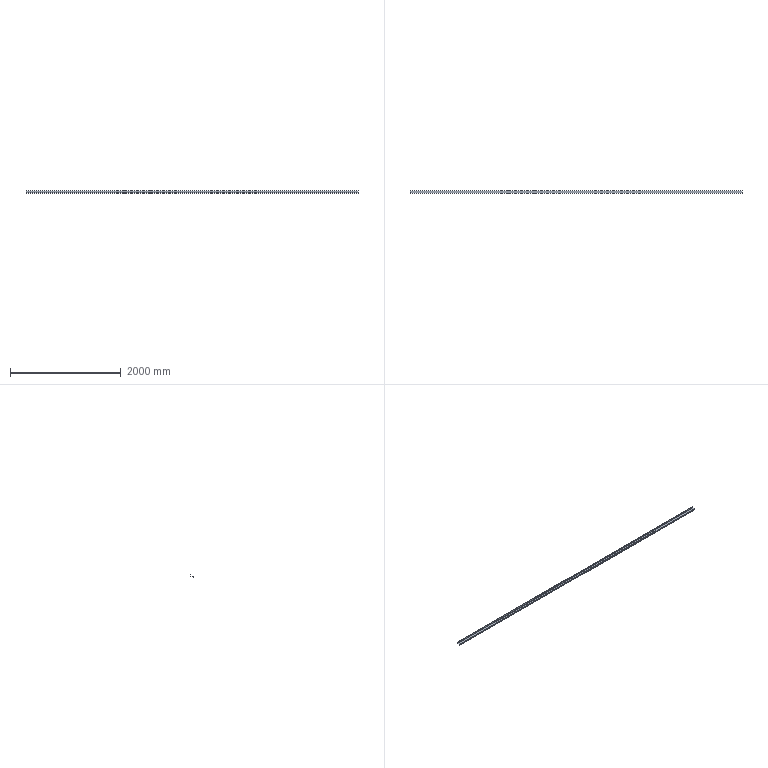Part | STEP file | Microwave Drying Flat Conveyor-CN2500x400-104-101_DefaultSM-FLAT-PATTERN | 1 solid | 22 faces | box 6000 x 50 x 47 mm | volume 1622469 mm3 | plane 18 | cylinder 4 | commonest cylinder face diameters 6 x2 12 x2
STEP:
#1=CARTESIAN_POINT('',(-3000.,19.,-3.));
#2=VERTEX_POINT('',#1);
#3=CARTESIAN_POINT('',(-3000.,-19.,-3.));
#4=VERTEX_POINT('',#3);
#5=CARTESIAN_POINT('',(-3000.,25.,-3.));
#6=DIRECTION('',(0.,-1.,0.));
#7=VECTOR('',#6,1000.);
#8=LINE('',#5,#7);
#9=EDGE_CURVE('',#2,#4,#8,.T.);
#10=ORIENTED_EDGE('',*,*,#9,.T.);
#11=CARTESIAN_POINT('',(-3000.,-19.,0.));
#12=VERTEX_POINT('',#11);
#13=CARTESIAN_POINT('',(-3000.,-19.,-3.));
#14=DIRECTION('',(0.,0.,1.));
#15=VECTOR('',#14,1000.);
#16=LINE('',#13,#15);
#17=EDGE_CURVE('',#4,#12,#16,.T.);
#18=ORIENTED_EDGE('',*,*,#17,.T.);
#19=CARTESIAN_POINT('',(-3000.,19.,0.));
#20=VERTEX_POINT('',#19);
#21=CARTESIAN_POINT('',(-3000.,25.,0.));
#22=DIRECTION('',(0.,-1.,0.));
#23=VECTOR('',#22,1000.);
#24=LINE('',#21,#23);
#25=EDGE_CURVE('',#20,#12,#24,.T.);
#26=ORIENTED_EDGE('',*,*,#25,.F.);
#27=CARTESIAN_POINT('',(-3000.,19.,0.));
#28=DIRECTION('',(0.,0.,-1.));
#29=VECTOR('',#28,1000.);
#30=LINE('',#27,#29);
#31=EDGE_CURVE('',#20,#2,#30,.T.);
#32=ORIENTED_EDGE('',*,*,#31,.T.);
#33=EDGE_LOOP('',(#10,#18,#26,#32));
#34=FACE_OUTER_BOUND('',#33,.T.);
#35=CARTESIAN_POINT('',(-3000.,25.,-3.));
#36=DIRECTION('',(-1.,0.,0.));
#37=DIRECTION('',(0.,0.,1.));
#38=AXIS2_PLACEMENT_3D('',#35,#36,#37);
#39=PLANE('',#38);
#40=ADVANCED_FACE('',(#34),#39,.T.);
#41=CARTESIAN_POINT('',(3000.,-19.,-3.));
#42=VERTEX_POINT('',#41);
#43=CARTESIAN_POINT('',(-3000.,-19.,-3.));
#44=DIRECTION('',(1.,0.,0.));
#45=VECTOR('',#44,1000.);
#46=LINE('',#43,#45);
#47=EDGE_CURVE('',#4,#42,#46,.T.);
#48=ORIENTED_EDGE('',*,*,#47,.F.);
#49=ORIENTED_EDGE('',*,*,#9,.F.);
#50=CARTESIAN_POINT('',(3000.,19.,-3.));
#51=VERTEX_POINT('',#50);
#52=CARTESIAN_POINT('',(-3000.,19.,-3.));
#53=DIRECTION('',(1.,0.,0.));
#54=VECTOR('',#53,1000.);
#55=LINE('',#52,#54);
#56=EDGE_CURVE('',#2,#51,#55,.T.);
#57=ORIENTED_EDGE('',*,*,#56,.T.);
#58=CARTESIAN_POINT('',(3000.,25.,-3.));
#59=DIRECTION('',(0.,1.,0.));
#60=VECTOR('',#59,1000.);
#61=LINE('',#58,#60);
#62=EDGE_CURVE('',#42,#51,#61,.T.);
#63=ORIENTED_EDGE('',*,*,#62,.F.);
#64=EDGE_LOOP('',(#48,#49,#57,#63));
#65=FACE_OUTER_BOUND('',#64,.T.);
#66=CARTESIAN_POINT('',(0.,0.,-3.));
#67=DIRECTION('',(0.,0.,1.));
#68=DIRECTION('',(1.,0.,0.));
#69=AXIS2_PLACEMENT_3D('',#66,#67,#68);
#70=PLANE('',#69);
#71=ADVANCED_FACE('',(#65),#70,.F.);
#72=ORIENTED_EDGE('',*,*,#25,.T.);
#73=CARTESIAN_POINT('',(3000.,-19.,0.));
#74=VERTEX_POINT('',#73);
#75=CARTESIAN_POINT('',(-3000.,-19.,0.));
#76=DIRECTION('',(1.,0.,0.));
#77=VECTOR('',#76,1000.);
#78=LINE('',#75,#77);
#79=EDGE_CURVE('',#12,#74,#78,.T.);
#80=ORIENTED_EDGE('',*,*,#79,.T.);
#81=CARTESIAN_POINT('',(3000.,19.,0.));
#82=VERTEX_POINT('',#81);
#83=CARTESIAN_POINT('',(3000.,25.,0.));
#84=DIRECTION('',(0.,1.,0.));
#85=VECTOR('',#84,1000.);
#86=LINE('',#83,#85);
#87=EDGE_CURVE('',#74,#82,#86,.T.);
#88=ORIENTED_EDGE('',*,*,#87,.T.);
#89=CARTESIAN_POINT('',(-3000.,19.,0.));
#90=DIRECTION('',(1.,0.,0.));
#91=VECTOR('',#90,1000.);
#92=LINE('',#89,#91);
#93=EDGE_CURVE('',#20,#82,#92,.T.);
#94=ORIENTED_EDGE('',*,*,#93,.F.);
#95=EDGE_LOOP('',(#72,#80,#88,#94));
#96=FACE_OUTER_BOUND('',#95,.T.);
#97=CARTESIAN_POINT('',(0.,0.,0.));
#98=DIRECTION('',(0.,0.,1.));
#99=DIRECTION('',(1.,0.,0.));
#100=AXIS2_PLACEMENT_3D('',#97,#98,#99);
#101=PLANE('',#100);
#102=ADVANCED_FACE('',(#96),#101,.T.);
#103=CARTESIAN_POINT('',(3000.,-19.,-3.));
#104=DIRECTION('',(0.,0.,1.));
#105=VECTOR('',#104,1000.);
#106=LINE('',#103,#105);
#107=EDGE_CURVE('',#42,#74,#106,.T.);
#108=ORIENTED_EDGE('',*,*,#107,.F.);
#109=ORIENTED_EDGE('',*,*,#62,.T.);
#110=CARTESIAN_POINT('',(3000.,19.,0.));
#111=DIRECTION('',(0.,0.,-1.));
#112=VECTOR('',#111,1000.);
#113=LINE('',#110,#112);
#114=EDGE_CURVE('',#82,#51,#113,.T.);
#115=ORIENTED_EDGE('',*,*,#114,.F.);
#116=ORIENTED_EDGE('',*,*,#87,.F.);
#117=EDGE_LOOP('',(#108,#109,#115,#116));
#118=FACE_OUTER_BOUND('',#117,.T.);
#119=CARTESIAN_POINT('',(3000.,25.,-3.));
#120=DIRECTION('',(1.,0.,0.));
#121=DIRECTION('',(0.,0.,-1.));
#122=AXIS2_PLACEMENT_3D('',#119,#120,#121);
#123=PLANE('',#122);
#124=ADVANCED_FACE('',(#118),#123,.T.);
#125=CARTESIAN_POINT('',(3000.,22.,3.));
#126=VERTEX_POINT('',#125);
#127=CARTESIAN_POINT('',(3000.,25.,3.));
#128=VERTEX_POINT('',#127);
#129=CARTESIAN_POINT('',(3000.,25.,3.));
#130=DIRECTION('',(0.,1.,0.));
#131=VECTOR('',#130,1000.);
#132=LINE('',#129,#131);
#133=EDGE_CURVE('',#126,#128,#132,.T.);
#134=ORIENTED_EDGE('',*,*,#133,.F.);
#135=CARTESIAN_POINT('',(3000.,19.,3.));
#136=DIRECTION('',(1.,0.,0.));
#137=DIRECTION('',(0.,0.,1.));
#138=AXIS2_PLACEMENT_3D('',#135,#136,#137);
#139=CIRCLE('',#138,3.);
#140=EDGE_CURVE('',#82,#126,#139,.T.);
#141=ORIENTED_EDGE('',*,*,#140,.F.);
#142=ORIENTED_EDGE('',*,*,#114,.T.);
#143=CARTESIAN_POINT('',(3000.,19.,3.));
#144=DIRECTION('',(1.,0.,0.));
#145=DIRECTION('',(0.,0.,1.));
#146=AXIS2_PLACEMENT_3D('',#143,#144,#145);
#147=CIRCLE('',#146,6.);
#148=EDGE_CURVE('',#51,#128,#147,.T.);
#149=ORIENTED_EDGE('',*,*,#148,.T.);
#150=EDGE_LOOP('',(#134,#141,#142,#149));
#151=FACE_OUTER_BOUND('',#150,.T.);
#152=CARTESIAN_POINT('',(3000.,19.,3.));
#153=DIRECTION('',(1.,0.,0.));
#154=DIRECTION('',(0.,0.,-1.));
#155=AXIS2_PLACEMENT_3D('',#152,#153,#154);
#156=PLANE('',#155);
#157=ADVANCED_FACE('',(#151),#156,.T.);
#158=CARTESIAN_POINT('',(-3000.,22.,3.));
#159=VERTEX_POINT('',#158);
#160=CARTESIAN_POINT('',(-3000.,19.,3.));
#161=DIRECTION('',(-1.,0.,0.));
#162=DIRECTION('',(0.,0.,1.));
#163=AXIS2_PLACEMENT_3D('',#160,#161,#162);
#164=CIRCLE('',#163,3.);
#165=EDGE_CURVE('',#159,#20,#164,.T.);
#166=ORIENTED_EDGE('',*,*,#165,.F.);
#167=CARTESIAN_POINT('',(-3000.,25.,3.));
#168=VERTEX_POINT('',#167);
#169=CARTESIAN_POINT('',(-3000.,22.,3.));
#170=DIRECTION('',(0.,1.,0.));
#171=VECTOR('',#170,1000.);
#172=LINE('',#169,#171);
#173=EDGE_CURVE('',#159,#168,#172,.T.);
#174=ORIENTED_EDGE('',*,*,#173,.T.);
#175=CARTESIAN_POINT('',(-3000.,19.,3.));
#176=DIRECTION('',(-1.,0.,0.));
#177=DIRECTION('',(0.,0.,1.));
#178=AXIS2_PLACEMENT_3D('',#175,#176,#177);
#179=CIRCLE('',#178,6.);
#180=EDGE_CURVE('',#168,#2,#179,.T.);
#181=ORIENTED_EDGE('',*,*,#180,.T.);
#182=ORIENTED_EDGE('',*,*,#31,.F.);
#183=EDGE_LOOP('',(#166,#174,#181,#182));
#184=FACE_OUTER_BOUND('',#183,.T.);
#185=CARTESIAN_POINT('',(-3000.,19.,3.));
#186=DIRECTION('',(1.,0.,0.));
#187=DIRECTION('',(0.,0.,-1.));
#188=AXIS2_PLACEMENT_3D('',#185,#186,#187);
#189=PLANE('',#188);
#190=ADVANCED_FACE('',(#184),#189,.F.);
#191=ORIENTED_EDGE('',*,*,#56,.F.);
#192=ORIENTED_EDGE('',*,*,#180,.F.);
#193=CARTESIAN_POINT('',(3000.,25.,3.));
#194=DIRECTION('',(1.,0.,0.));
#195=VECTOR('',#194,1000.);
#196=LINE('',#193,#195);
#197=EDGE_CURVE('',#168,#128,#196,.T.);
#198=ORIENTED_EDGE('',*,*,#197,.T.);
#199=ORIENTED_EDGE('',*,*,#148,.F.);
#200=EDGE_LOOP('',(#191,#192,#198,#199));
#201=FACE_OUTER_BOUND('',#200,.T.);
#202=CARTESIAN_POINT('',(-3000.,19.,3.));
#203=DIRECTION('',(-1.,0.,0.));
#204=DIRECTION('',(0.,1.,0.));
#205=AXIS2_PLACEMENT_3D('',#202,#203,#204);
#206=CYLINDRICAL_SURFACE('',#205,6.);
#207=ADVANCED_FACE('',(#201),#206,.T.);
#208=ORIENTED_EDGE('',*,*,#93,.T.);
#209=ORIENTED_EDGE('',*,*,#140,.T.);
#210=CARTESIAN_POINT('',(3000.,22.,3.));
#211=DIRECTION('',(-1.,0.,0.));
#212=VECTOR('',#211,1000.);
#213=LINE('',#210,#212);
#214=EDGE_CURVE('',#126,#159,#213,.T.);
#215=ORIENTED_EDGE('',*,*,#214,.T.);
#216=ORIENTED_EDGE('',*,*,#165,.T.);
#217=EDGE_LOOP('',(#208,#209,#215,#216));
#218=FACE_OUTER_BOUND('',#217,.T.);
#219=CARTESIAN_POINT('',(-3000.,19.,3.));
#220=DIRECTION('',(-1.,0.,0.));
#221=DIRECTION('',(0.,1.,0.));
#222=AXIS2_PLACEMENT_3D('',#219,#220,#221);
#223=CYLINDRICAL_SURFACE('',#222,3.);
#224=ADVANCED_FACE('',(#218),#223,.F.);
#225=ORIENTED_EDGE('',*,*,#173,.F.);
#226=CARTESIAN_POINT('',(-3000.,22.,27.));
#227=VERTEX_POINT('',#226);
#228=CARTESIAN_POINT('',(-3000.,22.,27.));
#229=DIRECTION('',(0.,0.,1.));
#230=VECTOR('',#229,1000.);
#231=LINE('',#228,#230);
#232=EDGE_CURVE('',#159,#227,#231,.T.);
#233=ORIENTED_EDGE('',*,*,#232,.T.);
#234=CARTESIAN_POINT('',(-3000.,25.,27.));
#235=VERTEX_POINT('',#234);
#236=CARTESIAN_POINT('',(-3000.,25.,27.));
#237=DIRECTION('',(0.,-1.,0.));
#238=VECTOR('',#237,1000.);
#239=LINE('',#236,#238);
#240=EDGE_CURVE('',#235,#227,#239,.T.);
#241=ORIENTED_EDGE('',*,*,#240,.F.);
#242=CARTESIAN_POINT('',(-3000.,25.,0.));
#243=DIRECTION('',(0.,0.,1.));
#244=VECTOR('',#243,1000.);
#245=LINE('',#242,#244);
#246=EDGE_CURVE('',#168,#235,#245,.T.);
#247=ORIENTED_EDGE('',*,*,#246,.F.);
#248=EDGE_LOOP('',(#225,#233,#241,#247));
#249=FACE_OUTER_BOUND('',#248,.T.);
#250=CARTESIAN_POINT('',(-3000.,25.,27.));
#251=DIRECTION('',(1.,0.,0.));
#252=DIRECTION('',(0.,0.,-1.));
#253=AXIS2_PLACEMENT_3D('',#250,#251,#252);
#254=PLANE('',#253);
#255=ADVANCED_FACE('',(#249),#254,.F.);
#256=ORIENTED_EDGE('',*,*,#133,.T.);
#257=CARTESIAN_POINT('',(3000.,25.,27.));
#258=VERTEX_POINT('',#257);
#259=CARTESIAN_POINT('',(3000.,25.,0.));
#260=DIRECTION('',(0.,0.,-1.));
#261=VECTOR('',#260,1000.);
#262=LINE('',#259,#261);
#263=EDGE_CURVE('',#258,#128,#262,.T.);
#264=ORIENTED_EDGE('',*,*,#263,.F.);
#265=CARTESIAN_POINT('',(3000.,22.,27.));
#266=VERTEX_POINT('',#265);
#267=CARTESIAN_POINT('',(3000.,25.,27.));
#268=DIRECTION('',(0.,-1.,0.));
#269=VECTOR('',#268,1000.);
#270=LINE('',#267,#269);
#271=EDGE_CURVE('',#258,#266,#270,.T.);
#272=ORIENTED_EDGE('',*,*,#271,.T.);
#273=CARTESIAN_POINT('',(3000.,22.,0.));
#274=DIRECTION('',(0.,0.,-1.));
#275=VECTOR('',#274,1000.);
#276=LINE('',#273,#275);
#277=EDGE_CURVE('',#266,#126,#276,.T.);
#278=ORIENTED_EDGE('',*,*,#277,.T.);
#279=EDGE_LOOP('',(#256,#264,#272,#278));
#280=FACE_OUTER_BOUND('',#279,.T.);
#281=CARTESIAN_POINT('',(3000.,25.,0.));
#282=DIRECTION('',(-1.,0.,0.));
#283=DIRECTION('',(0.,0.,1.));
#284=AXIS2_PLACEMENT_3D('',#281,#282,#283);
#285=PLANE('',#284);
#286=ADVANCED_FACE('',(#280),#285,.F.);
#287=ORIENTED_EDGE('',*,*,#197,.F.);
#288=ORIENTED_EDGE('',*,*,#246,.T.);
#289=CARTESIAN_POINT('',(0.,25.,27.));
#290=DIRECTION('',(1.,0.,0.));
#291=VECTOR('',#290,1000.);
#292=LINE('',#289,#291);
#293=EDGE_CURVE('',#235,#258,#292,.T.);
#294=ORIENTED_EDGE('',*,*,#293,.T.);
#295=ORIENTED_EDGE('',*,*,#263,.T.);
#296=EDGE_LOOP('',(#287,#288,#294,#295));
#297=FACE_OUTER_BOUND('',#296,.T.);
#298=CARTESIAN_POINT('',(0.,25.,0.));
#299=DIRECTION('',(0.,-1.,0.));
#300=DIRECTION('',(0.,0.,-1.));
#301=AXIS2_PLACEMENT_3D('',#298,#299,#300);
#302=PLANE('',#301);
#303=ADVANCED_FACE('',(#297),#302,.F.);
#304=ORIENTED_EDGE('',*,*,#232,.F.);
#305=ORIENTED_EDGE('',*,*,#214,.F.);
#306=ORIENTED_EDGE('',*,*,#277,.F.);
#307=CARTESIAN_POINT('',(3000.,22.,27.));
#308=DIRECTION('',(1.,0.,0.));
#309=VECTOR('',#308,1000.);
#310=LINE('',#307,#309);
#311=EDGE_CURVE('',#227,#266,#310,.T.);
#312=ORIENTED_EDGE('',*,*,#311,.F.);
#313=EDGE_LOOP('',(#304,#305,#306,#312));
#314=FACE_OUTER_BOUND('',#313,.T.);
#315=CARTESIAN_POINT('',(0.,22.,0.));
#316=DIRECTION('',(0.,-1.,0.));
#317=DIRECTION('',(0.,0.,-1.));
#318=AXIS2_PLACEMENT_3D('',#315,#316,#317);
#319=PLANE('',#318);
#320=ADVANCED_FACE('',(#314),#319,.T.);
#321=ORIENTED_EDGE('',*,*,#311,.T.);
#322=ORIENTED_EDGE('',*,*,#271,.F.);
#323=ORIENTED_EDGE('',*,*,#293,.F.);
#324=ORIENTED_EDGE('',*,*,#240,.T.);
#325=EDGE_LOOP('',(#321,#322,#323,#324));
#326=FACE_OUTER_BOUND('',#325,.T.);
#327=CARTESIAN_POINT('',(3000.,25.,27.));
#328=DIRECTION('',(0.,0.,-1.));
#329=DIRECTION('',(0.,1.,0.));
#330=AXIS2_PLACEMENT_3D('',#327,#328,#329);
#331=PLANE('',#330);
#332=ADVANCED_FACE('',(#326),#331,.F.);
#333=CARTESIAN_POINT('',(3000.,-22.,-6.));
#334=VERTEX_POINT('',#333);
#335=CARTESIAN_POINT('',(3000.,-25.,-6.));
#336=VERTEX_POINT('',#335);
#337=CARTESIAN_POINT('',(3000.,-25.,-6.));
#338=DIRECTION('',(0.,-1.,0.));
#339=VECTOR('',#338,1000.);
#340=LINE('',#337,#339);
#341=EDGE_CURVE('',#334,#336,#340,.T.);
#342=ORIENTED_EDGE('',*,*,#341,.F.);
#343=CARTESIAN_POINT('',(3000.,-19.,-6.));
#344=DIRECTION('',(1.,0.,0.));
#345=DIRECTION('',(0.,0.,1.));
#346=AXIS2_PLACEMENT_3D('',#343,#344,#345);
#347=CIRCLE('',#346,3.);
#348=EDGE_CURVE('',#42,#334,#347,.T.);
#349=ORIENTED_EDGE('',*,*,#348,.F.);
#350=ORIENTED_EDGE('',*,*,#107,.T.);
#351=CARTESIAN_POINT('',(3000.,-19.,-6.));
#352=DIRECTION('',(1.,0.,0.));
#353=DIRECTION('',(0.,0.,1.));
#354=AXIS2_PLACEMENT_3D('',#351,#352,#353);
#355=CIRCLE('',#354,6.);
#356=EDGE_CURVE('',#74,#336,#355,.T.);
#357=ORIENTED_EDGE('',*,*,#356,.T.);
#358=EDGE_LOOP('',(#342,#349,#350,#357));
#359=FACE_OUTER_BOUND('',#358,.T.);
#360=CARTESIAN_POINT('',(3000.,-19.,-6.));
#361=DIRECTION('',(1.,0.,0.));
#362=DIRECTION('',(0.,0.,-1.));
#363=AXIS2_PLACEMENT_3D('',#360,#361,#362);
#364=PLANE('',#363);
#365=ADVANCED_FACE('',(#359),#364,.T.);
#366=CARTESIAN_POINT('',(-3000.,-22.,-6.));
#367=VERTEX_POINT('',#366);
#368=CARTESIAN_POINT('',(-3000.,-19.,-6.));
#369=DIRECTION('',(-1.,0.,0.));
#370=DIRECTION('',(0.,0.,1.));
#371=AXIS2_PLACEMENT_3D('',#368,#369,#370);
#372=CIRCLE('',#371,3.);
#373=EDGE_CURVE('',#367,#4,#372,.T.);
#374=ORIENTED_EDGE('',*,*,#373,.F.);
#375=CARTESIAN_POINT('',(-3000.,-25.,-6.));
#376=VERTEX_POINT('',#375);
#377=CARTESIAN_POINT('',(-3000.,-22.,-6.));
#378=DIRECTION('',(0.,-1.,0.));
#379=VECTOR('',#378,1000.);
#380=LINE('',#377,#379);
#381=EDGE_CURVE('',#367,#376,#380,.T.);
#382=ORIENTED_EDGE('',*,*,#381,.T.);
#383=CARTESIAN_POINT('',(-3000.,-19.,-6.));
#384=DIRECTION('',(-1.,0.,0.));
#385=DIRECTION('',(0.,0.,1.));
#386=AXIS2_PLACEMENT_3D('',#383,#384,#385);
#387=CIRCLE('',#386,6.);
#388=EDGE_CURVE('',#376,#12,#387,.T.);
#389=ORIENTED_EDGE('',*,*,#388,.T.);
#390=ORIENTED_EDGE('',*,*,#17,.F.);
#391=EDGE_LOOP('',(#374,#382,#389,#390));
#392=FACE_OUTER_BOUND('',#391,.T.);
#393=CARTESIAN_POINT('',(-3000.,-19.,-6.));
#394=DIRECTION('',(1.,0.,0.));
#395=DIRECTION('',(0.,0.,-1.));
#396=AXIS2_PLACEMENT_3D('',#393,#394,#395);
#397=PLANE('',#396);
#398=ADVANCED_FACE('',(#392),#397,.F.);
#399=ORIENTED_EDGE('',*,*,#79,.F.);
#400=ORIENTED_EDGE('',*,*,#388,.F.);
#401=CARTESIAN_POINT('',(0.,-25.,-6.));
#402=DIRECTION('',(-1.,0.,0.));
#403=VECTOR('',#402,1000.);
#404=LINE('',#401,#403);
#405=EDGE_CURVE('',#336,#376,#404,.T.);
#406=ORIENTED_EDGE('',*,*,#405,.F.);
#407=ORIENTED_EDGE('',*,*,#356,.F.);
#408=EDGE_LOOP('',(#399,#400,#406,#407));
#409=FACE_OUTER_BOUND('',#408,.T.);
#410=CARTESIAN_POINT('',(-3000.,-19.,-6.));
#411=DIRECTION('',(-1.,0.,0.));
#412=DIRECTION('',(0.,-1.,0.));
#413=AXIS2_PLACEMENT_3D('',#410,#411,#412);
#414=CYLINDRICAL_SURFACE('',#413,6.);
#415=ADVANCED_FACE('',(#409),#414,.T.);
#416=ORIENTED_EDGE('',*,*,#47,.T.);
#417=ORIENTED_EDGE('',*,*,#348,.T.);
#418=CARTESIAN_POINT('',(3000.,-22.,-6.));
#419=DIRECTION('',(-1.,0.,0.));
#420=VECTOR('',#419,1000.);
#421=LINE('',#418,#420);
#422=EDGE_CURVE('',#334,#367,#421,.T.);
#423=ORIENTED_EDGE('',*,*,#422,.T.);
#424=ORIENTED_EDGE('',*,*,#373,.T.);
#425=EDGE_LOOP('',(#416,#417,#423,#424));
#426=FACE_OUTER_BOUND('',#425,.T.);
#427=CARTESIAN_POINT('',(-3000.,-19.,-6.));
#428=DIRECTION('',(-1.,0.,0.));
#429=DIRECTION('',(0.,-1.,0.));
#430=AXIS2_PLACEMENT_3D('',#427,#428,#429);
#431=CYLINDRICAL_SURFACE('',#430,3.);
#432=ADVANCED_FACE('',(#426),#431,.F.);
#433=CARTESIAN_POINT('',(-3000.,-25.,-20.));
#434=VERTEX_POINT('',#433);
#435=CARTESIAN_POINT('',(-3000.,-25.,-3.));
#436=DIRECTION('',(0.,0.,1.));
#437=VECTOR('',#436,1000.);
#438=LINE('',#435,#437);
#439=EDGE_CURVE('',#434,#376,#438,.T.);
#440=ORIENTED_EDGE('',*,*,#439,.T.);
#441=ORIENTED_EDGE('',*,*,#381,.F.);
#442=CARTESIAN_POINT('',(-3000.,-22.,-20.));
#443=VERTEX_POINT('',#442);
#444=CARTESIAN_POINT('',(-3000.,-22.,0.));
#445=DIRECTION('',(0.,0.,1.));
#446=VECTOR('',#445,1000.);
#447=LINE('',#444,#446);
#448=EDGE_CURVE('',#443,#367,#447,.T.);
#449=ORIENTED_EDGE('',*,*,#448,.F.);
#450=CARTESIAN_POINT('',(-3000.,-25.,-20.));
#451=DIRECTION('',(0.,1.,0.));
#452=VECTOR('',#451,1000.);
#453=LINE('',#450,#452);
#454=EDGE_CURVE('',#434,#443,#453,.T.);
#455=ORIENTED_EDGE('',*,*,#454,.F.);
#456=EDGE_LOOP('',(#440,#441,#449,#455));
#457=FACE_OUTER_BOUND('',#456,.T.);
#458=CARTESIAN_POINT('',(-3000.,-25.,-3.));
#459=DIRECTION('',(-1.,0.,0.));
#460=DIRECTION('',(0.,0.,1.));
#461=AXIS2_PLACEMENT_3D('',#458,#459,#460);
#462=PLANE('',#461);
#463=ADVANCED_FACE('',(#457),#462,.T.);
#464=CARTESIAN_POINT('',(3000.,-22.,-20.));
#465=VERTEX_POINT('',#464);
#466=CARTESIAN_POINT('',(3000.,-22.,0.));
#467=DIRECTION('',(0.,0.,-1.));
#468=VECTOR('',#467,1000.);
#469=LINE('',#466,#468);
#470=EDGE_CURVE('',#334,#465,#469,.T.);
#471=ORIENTED_EDGE('',*,*,#470,.F.);
#472=ORIENTED_EDGE('',*,*,#341,.T.);
#473=CARTESIAN_POINT('',(3000.,-25.,-20.));
#474=VERTEX_POINT('',#473);
#475=CARTESIAN_POINT('',(3000.,-25.,-20.));
#476=DIRECTION('',(0.,0.,-1.));
#477=VECTOR('',#476,1000.);
#478=LINE('',#475,#477);
#479=EDGE_CURVE('',#336,#474,#478,.T.);
#480=ORIENTED_EDGE('',*,*,#479,.T.);
#481=CARTESIAN_POINT('',(3000.,-25.,-20.));
#482=DIRECTION('',(0.,1.,0.));
#483=VECTOR('',#482,1000.);
#484=LINE('',#481,#483);
#485=EDGE_CURVE('',#474,#465,#484,.T.);
#486=ORIENTED_EDGE('',*,*,#485,.T.);
#487=EDGE_LOOP('',(#471,#472,#480,#486));
#488=FACE_OUTER_BOUND('',#487,.T.);
#489=CARTESIAN_POINT('',(3000.,-25.,-20.));
#490=DIRECTION('',(1.,0.,0.));
#491=DIRECTION('',(0.,0.,-1.));
#492=AXIS2_PLACEMENT_3D('',#489,#490,#491);
#493=PLANE('',#492);
#494=ADVANCED_FACE('',(#488),#493,.T.);
#495=ORIENTED_EDGE('',*,*,#479,.F.);
#496=ORIENTED_EDGE('',*,*,#405,.T.);
#497=ORIENTED_EDGE('',*,*,#439,.F.);
#498=CARTESIAN_POINT('',(-3000.,-25.,-20.));
#499=DIRECTION('',(-1.,0.,0.));
#500=VECTOR('',#499,1000.);
#501=LINE('',#498,#500);
#502=EDGE_CURVE('',#474,#434,#501,.T.);
#503=ORIENTED_EDGE('',*,*,#502,.F.);
#504=EDGE_LOOP('',(#495,#496,#497,#503));
#505=FACE_OUTER_BOUND('',#504,.T.);
#506=CARTESIAN_POINT('',(0.,-25.,0.));
#507=DIRECTION('',(0.,-1.,0.));
#508=DIRECTION('',(0.,0.,-1.));
#509=AXIS2_PLACEMENT_3D('',#506,#507,#508);
#510=PLANE('',#509);
#511=ADVANCED_FACE('',(#505),#510,.T.);
#512=ORIENTED_EDGE('',*,*,#422,.F.);
#513=ORIENTED_EDGE('',*,*,#470,.T.);
#514=CARTESIAN_POINT('',(0.,-22.,-20.));
#515=DIRECTION('',(-1.,0.,0.));
#516=VECTOR('',#515,1000.);
#517=LINE('',#514,#516);
#518=EDGE_CURVE('',#465,#443,#517,.T.);
#519=ORIENTED_EDGE('',*,*,#518,.T.);
#520=ORIENTED_EDGE('',*,*,#448,.T.);
#521=EDGE_LOOP('',(#512,#513,#519,#520));
#522=FACE_OUTER_BOUND('',#521,.T.);
#523=CARTESIAN_POINT('',(0.,-22.,0.));
#524=DIRECTION('',(0.,-1.,0.));
#525=DIRECTION('',(0.,0.,-1.));
#526=AXIS2_PLACEMENT_3D('',#523,#524,#525);
#527=PLANE('',#526);
#528=ADVANCED_FACE('',(#522),#527,.F.);
#529=ORIENTED_EDGE('',*,*,#518,.F.);
#530=ORIENTED_EDGE('',*,*,#485,.F.);
#531=ORIENTED_EDGE('',*,*,#502,.T.);
#532=ORIENTED_EDGE('',*,*,#454,.T.);
#533=EDGE_LOOP('',(#529,#530,#531,#532));
#534=FACE_OUTER_BOUND('',#533,.T.);
#535=CARTESIAN_POINT('',(-3000.,-25.,-20.));
#536=DIRECTION('',(0.,0.,-1.));
#537=DIRECTION('',(0.,1.,0.));
#538=AXIS2_PLACEMENT_3D('',#535,#536,#537);
#539=PLANE('',#538);
#540=ADVANCED_FACE('',(#534),#539,.T.);
#541=CLOSED_SHELL('',(#40,#71,#102,#124,#157,#190,#207,#224,#255,#286,#303,#320,#332,#365,#398,#415,#432,#463,#494,#511,#528,#540));
#542=MANIFOLD_SOLID_BREP('',#541);
#543=CARTESIAN_POINT('',(0.,0.,0.));
#544=DIRECTION('',(0.,0.,1.));
#545=DIRECTION('',(1.,0.,0.));
#546=AXIS2_PLACEMENT_3D('',#543,#544,#545);
#547=(LENGTH_UNIT()NAMED_UNIT(*)SI_UNIT(.MILLI.,.METRE.));
#548=UNCERTAINTY_MEASURE_WITH_UNIT(LENGTH_MEASURE(0.00001),#547,'','');
#549=(NAMED_UNIT(*)PLANE_ANGLE_UNIT()SI_UNIT($,.RADIAN.));
#550=(NAMED_UNIT(*)SI_UNIT($,.STERADIAN.)SOLID_ANGLE_UNIT());
#551=(GEOMETRIC_REPRESENTATION_CONTEXT(3)GLOBAL_UNCERTAINTY_ASSIGNED_CONTEXT((#548))GLOBAL_UNIT_ASSIGNED_CONTEXT((#547,#549,#550))REPRESENTATION_CONTEXT('',''));
#552=ADVANCED_BREP_SHAPE_REPRESENTATION('',(#542,#546),#551);